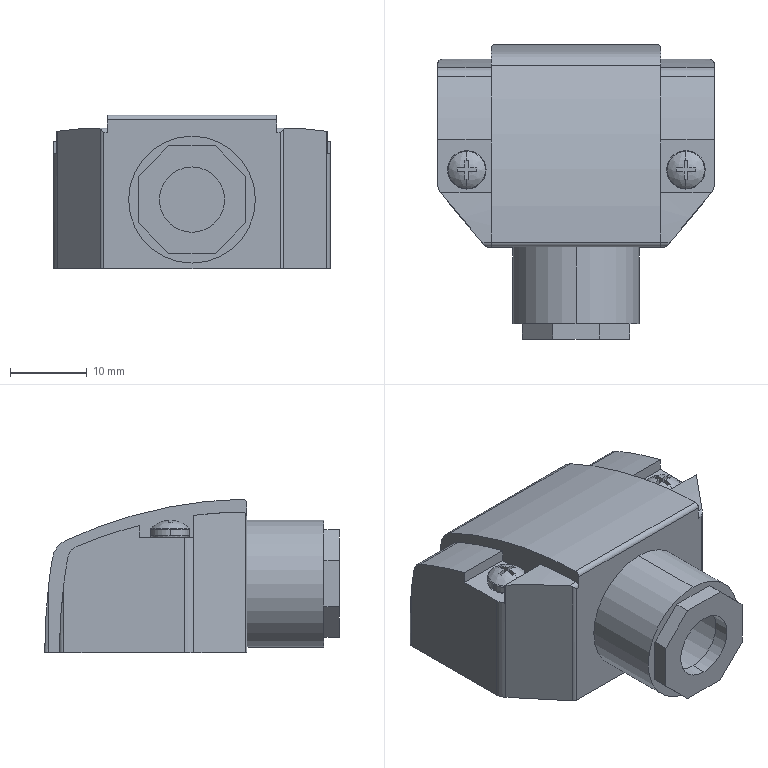Part | SolidWorks | features BaseBody 1 | 1 solid | 102 faces | box 36 x 38.3 x 19.99 mm | volume 14358 mm3 | plane 54 | cylinder 36 | spline 12 | commonest cylinder face diameters 1.2 x9 3.3 x4 5 x4 113.6 x4 150 x3 3.6 x2